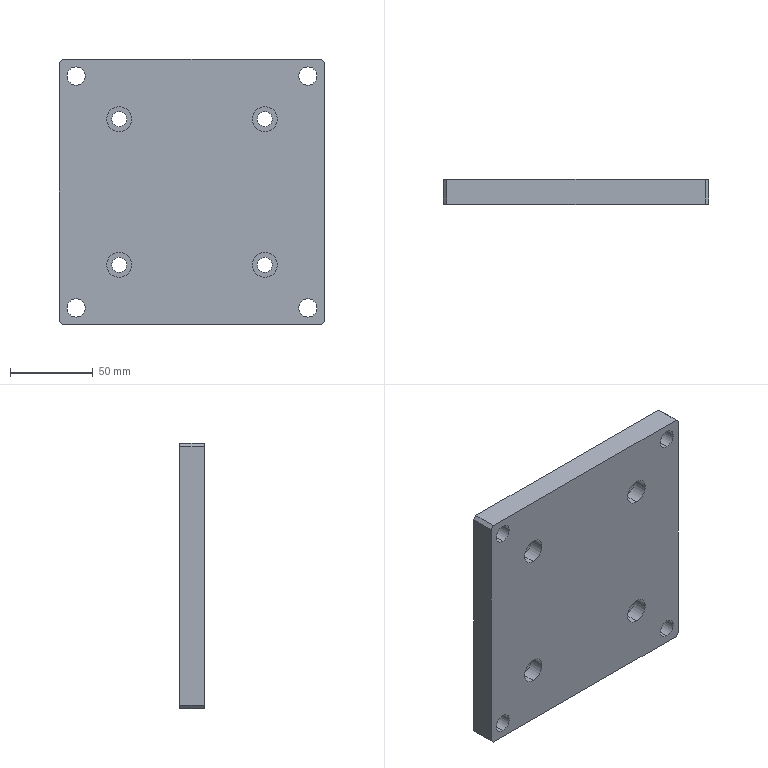Part | SolidWorks | features HoleWzd 2, Chamfer 1, Extrusion 1 | 1 solid | 38 faces | box 160 x 15 x 160 mm | volume 370289 mm3 | cylinder 24 | plane 14 | commonest cylinder face diameters 9 x8 11 x8 15 x8
STEP:
#1=CARTESIAN_POINT('',(70.,-7.5,64.5));
#2=VERTEX_POINT('',#1);
#3=CARTESIAN_POINT('',(70.,-7.5,75.5));
#4=VERTEX_POINT('',#3);
#5=CARTESIAN_POINT('',(70.,-7.5,70.));
#6=DIRECTION('',(0.,1.,0.));
#7=DIRECTION('',(0.,0.,1.));
#8=AXIS2_PLACEMENT_3D('',#5,#6,#7);
#9=CIRCLE('',#8,5.5);
#10=EDGE_CURVE('',#2,#4,#9,.T.);
#11=ORIENTED_EDGE('',*,*,#10,.F.);
#12=CARTESIAN_POINT('',(70.,7.5,64.5));
#13=VERTEX_POINT('',#12);
#14=CARTESIAN_POINT('',(70.,7.5,64.5));
#15=DIRECTION('',(0.,1.,0.));
#16=VECTOR('',#15,1000.);
#17=LINE('',#14,#16);
#18=EDGE_CURVE('',#2,#13,#17,.T.);
#19=ORIENTED_EDGE('',*,*,#18,.T.);
#20=CARTESIAN_POINT('',(70.,7.5,75.5));
#21=VERTEX_POINT('',#20);
#22=CARTESIAN_POINT('',(70.,7.5,70.));
#23=DIRECTION('',(0.,1.,0.));
#24=DIRECTION('',(0.,0.,1.));
#25=AXIS2_PLACEMENT_3D('',#22,#23,#24);
#26=CIRCLE('',#25,5.5);
#27=EDGE_CURVE('',#13,#21,#26,.T.);
#28=ORIENTED_EDGE('',*,*,#27,.T.);
#29=CARTESIAN_POINT('',(70.,7.5,75.5));
#30=DIRECTION('',(0.,1.,0.));
#31=VECTOR('',#30,1000.);
#32=LINE('',#29,#31);
#33=EDGE_CURVE('',#4,#21,#32,.T.);
#34=ORIENTED_EDGE('',*,*,#33,.F.);
#35=EDGE_LOOP('',(#11,#19,#28,#34));
#36=FACE_OUTER_BOUND('',#35,.T.);
#37=CARTESIAN_POINT('',(70.,7.5,70.));
#38=DIRECTION('',(0.,1.,0.));
#39=DIRECTION('',(0.,0.,1.));
#40=AXIS2_PLACEMENT_3D('',#37,#38,#39);
#41=CYLINDRICAL_SURFACE('',#40,5.5);
#42=ADVANCED_FACE('',(#36),#41,.F.);
#43=CARTESIAN_POINT('',(70.,-7.5,-75.5));
#44=VERTEX_POINT('',#43);
#45=CARTESIAN_POINT('',(70.,-7.5,-64.5));
#46=VERTEX_POINT('',#45);
#47=CARTESIAN_POINT('',(70.,-7.5,-70.));
#48=DIRECTION('',(0.,1.,0.));
#49=DIRECTION('',(0.,0.,1.));
#50=AXIS2_PLACEMENT_3D('',#47,#48,#49);
#51=CIRCLE('',#50,5.5);
#52=EDGE_CURVE('',#44,#46,#51,.T.);
#53=ORIENTED_EDGE('',*,*,#52,.F.);
#54=CARTESIAN_POINT('',(70.,7.5,-75.5));
#55=VERTEX_POINT('',#54);
#56=CARTESIAN_POINT('',(70.,7.5,-75.5));
#57=DIRECTION('',(0.,1.,0.));
#58=VECTOR('',#57,1000.);
#59=LINE('',#56,#58);
#60=EDGE_CURVE('',#44,#55,#59,.T.);
#61=ORIENTED_EDGE('',*,*,#60,.T.);
#62=CARTESIAN_POINT('',(70.,7.5,-64.5));
#63=VERTEX_POINT('',#62);
#64=CARTESIAN_POINT('',(70.,7.5,-70.));
#65=DIRECTION('',(0.,1.,0.));
#66=DIRECTION('',(0.,0.,1.));
#67=AXIS2_PLACEMENT_3D('',#64,#65,#66);
#68=CIRCLE('',#67,5.5);
#69=EDGE_CURVE('',#55,#63,#68,.T.);
#70=ORIENTED_EDGE('',*,*,#69,.T.);
#71=CARTESIAN_POINT('',(70.,7.5,-64.5));
#72=DIRECTION('',(0.,1.,0.));
#73=VECTOR('',#72,1000.);
#74=LINE('',#71,#73);
#75=EDGE_CURVE('',#46,#63,#74,.T.);
#76=ORIENTED_EDGE('',*,*,#75,.F.);
#77=EDGE_LOOP('',(#53,#61,#70,#76));
#78=FACE_OUTER_BOUND('',#77,.T.);
#79=CARTESIAN_POINT('',(70.,7.5,-70.));
#80=DIRECTION('',(0.,1.,0.));
#81=DIRECTION('',(0.,0.,1.));
#82=AXIS2_PLACEMENT_3D('',#79,#80,#81);
#83=CYLINDRICAL_SURFACE('',#82,5.5);
#84=ADVANCED_FACE('',(#78),#83,.F.);
#85=CARTESIAN_POINT('',(-70.,-7.5,-75.5));
#86=VERTEX_POINT('',#85);
#87=CARTESIAN_POINT('',(-70.,-7.5,-64.5));
#88=VERTEX_POINT('',#87);
#89=CARTESIAN_POINT('',(-70.,-7.5,-70.));
#90=DIRECTION('',(0.,1.,0.));
#91=DIRECTION('',(0.,0.,1.));
#92=AXIS2_PLACEMENT_3D('',#89,#90,#91);
#93=CIRCLE('',#92,5.5);
#94=EDGE_CURVE('',#86,#88,#93,.T.);
#95=ORIENTED_EDGE('',*,*,#94,.F.);
#96=CARTESIAN_POINT('',(-70.,7.5,-75.5));
#97=VERTEX_POINT('',#96);
#98=CARTESIAN_POINT('',(-70.,7.5,-75.5));
#99=DIRECTION('',(0.,1.,0.));
#100=VECTOR('',#99,1000.);
#101=LINE('',#98,#100);
#102=EDGE_CURVE('',#86,#97,#101,.T.);
#103=ORIENTED_EDGE('',*,*,#102,.T.);
#104=CARTESIAN_POINT('',(-70.,7.5,-64.5));
#105=VERTEX_POINT('',#104);
#106=CARTESIAN_POINT('',(-70.,7.5,-70.));
#107=DIRECTION('',(0.,1.,0.));
#108=DIRECTION('',(0.,0.,1.));
#109=AXIS2_PLACEMENT_3D('',#106,#107,#108);
#110=CIRCLE('',#109,5.5);
#111=EDGE_CURVE('',#97,#105,#110,.T.);
#112=ORIENTED_EDGE('',*,*,#111,.T.);
#113=CARTESIAN_POINT('',(-70.,7.5,-64.5));
#114=DIRECTION('',(0.,1.,0.));
#115=VECTOR('',#114,1000.);
#116=LINE('',#113,#115);
#117=EDGE_CURVE('',#88,#105,#116,.T.);
#118=ORIENTED_EDGE('',*,*,#117,.F.);
#119=EDGE_LOOP('',(#95,#103,#112,#118));
#120=FACE_OUTER_BOUND('',#119,.T.);
#121=CARTESIAN_POINT('',(-70.,7.5,-70.));
#122=DIRECTION('',(0.,1.,0.));
#123=DIRECTION('',(0.,0.,1.));
#124=AXIS2_PLACEMENT_3D('',#121,#122,#123);
#125=CYLINDRICAL_SURFACE('',#124,5.5);
#126=ADVANCED_FACE('',(#120),#125,.F.);
#127=CARTESIAN_POINT('',(-70.,-7.5,64.5));
#128=VERTEX_POINT('',#127);
#129=CARTESIAN_POINT('',(-70.,-7.5,75.5));
#130=VERTEX_POINT('',#129);
#131=CARTESIAN_POINT('',(-70.,-7.5,70.));
#132=DIRECTION('',(0.,1.,0.));
#133=DIRECTION('',(0.,0.,1.));
#134=AXIS2_PLACEMENT_3D('',#131,#132,#133);
#135=CIRCLE('',#134,5.5);
#136=EDGE_CURVE('',#128,#130,#135,.T.);
#137=ORIENTED_EDGE('',*,*,#136,.F.);
#138=CARTESIAN_POINT('',(-70.,7.5,64.5));
#139=VERTEX_POINT('',#138);
#140=CARTESIAN_POINT('',(-70.,7.5,64.5));
#141=DIRECTION('',(0.,1.,0.));
#142=VECTOR('',#141,1000.);
#143=LINE('',#140,#142);
#144=EDGE_CURVE('',#128,#139,#143,.T.);
#145=ORIENTED_EDGE('',*,*,#144,.T.);
#146=CARTESIAN_POINT('',(-70.,7.5,75.5));
#147=VERTEX_POINT('',#146);
#148=CARTESIAN_POINT('',(-70.,7.5,70.));
#149=DIRECTION('',(0.,1.,0.));
#150=DIRECTION('',(0.,0.,1.));
#151=AXIS2_PLACEMENT_3D('',#148,#149,#150);
#152=CIRCLE('',#151,5.5);
#153=EDGE_CURVE('',#139,#147,#152,.T.);
#154=ORIENTED_EDGE('',*,*,#153,.T.);
#155=CARTESIAN_POINT('',(-70.,7.5,75.5));
#156=DIRECTION('',(0.,1.,0.));
#157=VECTOR('',#156,1000.);
#158=LINE('',#155,#157);
#159=EDGE_CURVE('',#130,#147,#158,.T.);
#160=ORIENTED_EDGE('',*,*,#159,.F.);
#161=EDGE_LOOP('',(#137,#145,#154,#160));
#162=FACE_OUTER_BOUND('',#161,.T.);
#163=CARTESIAN_POINT('',(-70.,7.5,70.));
#164=DIRECTION('',(0.,1.,0.));
#165=DIRECTION('',(0.,0.,1.));
#166=AXIS2_PLACEMENT_3D('',#163,#164,#165);
#167=CYLINDRICAL_SURFACE('',#166,5.5);
#168=ADVANCED_FACE('',(#162),#167,.F.);
#169=CARTESIAN_POINT('',(-44.,1.5,51.5));
#170=VERTEX_POINT('',#169);
#171=CARTESIAN_POINT('',(-44.,1.5,36.5));
#172=VERTEX_POINT('',#171);
#173=CARTESIAN_POINT('',(-44.,1.5,44.));
#174=DIRECTION('',(0.,-1.,0.));
#175=DIRECTION('',(0.,0.,-1.));
#176=AXIS2_PLACEMENT_3D('',#173,#174,#175);
#177=CIRCLE('',#176,7.5);
#178=EDGE_CURVE('',#170,#172,#177,.T.);
#179=ORIENTED_EDGE('',*,*,#178,.F.);
#180=CARTESIAN_POINT('',(-44.,-7.5,51.5));
#181=VERTEX_POINT('',#180);
#182=CARTESIAN_POINT('',(-44.,-7.5,51.5));
#183=DIRECTION('',(0.,-1.,0.));
#184=VECTOR('',#183,1000.);
#185=LINE('',#182,#184);
#186=EDGE_CURVE('',#170,#181,#185,.T.);
#187=ORIENTED_EDGE('',*,*,#186,.T.);
#188=CARTESIAN_POINT('',(-44.,-7.5,36.5));
#189=VERTEX_POINT('',#188);
#190=CARTESIAN_POINT('',(-44.,-7.5,44.));
#191=DIRECTION('',(0.,-1.,0.));
#192=DIRECTION('',(0.,0.,-1.));
#193=AXIS2_PLACEMENT_3D('',#190,#191,#192);
#194=CIRCLE('',#193,7.5);
#195=EDGE_CURVE('',#181,#189,#194,.T.);
#196=ORIENTED_EDGE('',*,*,#195,.T.);
#197=CARTESIAN_POINT('',(-44.,-7.5,36.5));
#198=DIRECTION('',(0.,-1.,0.));
#199=VECTOR('',#198,1000.);
#200=LINE('',#197,#199);
#201=EDGE_CURVE('',#172,#189,#200,.T.);
#202=ORIENTED_EDGE('',*,*,#201,.F.);
#203=EDGE_LOOP('',(#179,#187,#196,#202));
#204=FACE_OUTER_BOUND('',#203,.T.);
#205=CARTESIAN_POINT('',(-44.,-7.5,44.));
#206=DIRECTION('',(0.,-1.,0.));
#207=DIRECTION('',(0.,0.,-1.));
#208=AXIS2_PLACEMENT_3D('',#205,#206,#207);
#209=CYLINDRICAL_SURFACE('',#208,7.5);
#210=ADVANCED_FACE('',(#204),#209,.F.);
#211=CARTESIAN_POINT('',(-44.,7.5,48.5));
#212=VERTEX_POINT('',#211);
#213=CARTESIAN_POINT('',(-44.,7.5,39.5));
#214=VERTEX_POINT('',#213);
#215=CARTESIAN_POINT('',(-44.,7.5,44.));
#216=DIRECTION('',(0.,-1.,0.));
#217=DIRECTION('',(0.,0.,-1.));
#218=AXIS2_PLACEMENT_3D('',#215,#216,#217);
#219=CIRCLE('',#218,4.5);
#220=EDGE_CURVE('',#212,#214,#219,.T.);
#221=ORIENTED_EDGE('',*,*,#220,.F.);
#222=CARTESIAN_POINT('',(-44.,1.5,48.5));
#223=VERTEX_POINT('',#222);
#224=CARTESIAN_POINT('',(-44.,-7.5,48.5));
#225=DIRECTION('',(0.,-1.,0.));
#226=VECTOR('',#225,1000.);
#227=LINE('',#224,#226);
#228=EDGE_CURVE('',#212,#223,#227,.T.);
#229=ORIENTED_EDGE('',*,*,#228,.T.);
#230=CARTESIAN_POINT('',(-44.,1.5,39.5));
#231=VERTEX_POINT('',#230);
#232=CARTESIAN_POINT('',(-44.,1.5,44.));
#233=DIRECTION('',(0.,-1.,0.));
#234=DIRECTION('',(0.,0.,-1.));
#235=AXIS2_PLACEMENT_3D('',#232,#233,#234);
#236=CIRCLE('',#235,4.5);
#237=EDGE_CURVE('',#223,#231,#236,.T.);
#238=ORIENTED_EDGE('',*,*,#237,.T.);
#239=CARTESIAN_POINT('',(-44.,-7.5,39.5));
#240=DIRECTION('',(0.,-1.,0.));
#241=VECTOR('',#240,1000.);
#242=LINE('',#239,#241);
#243=EDGE_CURVE('',#214,#231,#242,.T.);
#244=ORIENTED_EDGE('',*,*,#243,.F.);
#245=EDGE_LOOP('',(#221,#229,#238,#244));
#246=FACE_OUTER_BOUND('',#245,.T.);
#247=CARTESIAN_POINT('',(-44.,-7.5,44.));
#248=DIRECTION('',(0.,-1.,0.));
#249=DIRECTION('',(0.,0.,-1.));
#250=AXIS2_PLACEMENT_3D('',#247,#248,#249);
#251=CYLINDRICAL_SURFACE('',#250,4.5);
#252=ADVANCED_FACE('',(#246),#251,.F.);
#253=CARTESIAN_POINT('',(-44.,1.5,-36.5));
#254=VERTEX_POINT('',#253);
#255=CARTESIAN_POINT('',(-44.,1.5,-51.5));
#256=VERTEX_POINT('',#255);
#257=CARTESIAN_POINT('',(-44.,1.5,-44.));
#258=DIRECTION('',(0.,-1.,0.));
#259=DIRECTION('',(0.,0.,-1.));
#260=AXIS2_PLACEMENT_3D('',#257,#258,#259);
#261=CIRCLE('',#260,7.5);
#262=EDGE_CURVE('',#254,#256,#261,.T.);
#263=ORIENTED_EDGE('',*,*,#262,.F.);
#264=CARTESIAN_POINT('',(-44.,-7.5,-36.5));
#265=VERTEX_POINT('',#264);
#266=CARTESIAN_POINT('',(-44.,-7.5,-36.5));
#267=DIRECTION('',(0.,-1.,0.));
#268=VECTOR('',#267,1000.);
#269=LINE('',#266,#268);
#270=EDGE_CURVE('',#254,#265,#269,.T.);
#271=ORIENTED_EDGE('',*,*,#270,.T.);
#272=CARTESIAN_POINT('',(-44.,-7.5,-51.5));
#273=VERTEX_POINT('',#272);
#274=CARTESIAN_POINT('',(-44.,-7.5,-44.));
#275=DIRECTION('',(0.,-1.,0.));
#276=DIRECTION('',(0.,0.,-1.));
#277=AXIS2_PLACEMENT_3D('',#274,#275,#276);
#278=CIRCLE('',#277,7.5);
#279=EDGE_CURVE('',#265,#273,#278,.T.);
#280=ORIENTED_EDGE('',*,*,#279,.T.);
#281=CARTESIAN_POINT('',(-44.,-7.5,-51.5));
#282=DIRECTION('',(0.,-1.,0.));
#283=VECTOR('',#282,1000.);
#284=LINE('',#281,#283);
#285=EDGE_CURVE('',#256,#273,#284,.T.);
#286=ORIENTED_EDGE('',*,*,#285,.F.);
#287=EDGE_LOOP('',(#263,#271,#280,#286));
#288=FACE_OUTER_BOUND('',#287,.T.);
#289=CARTESIAN_POINT('',(-44.,-7.5,-44.));
#290=DIRECTION('',(0.,-1.,0.));
#291=DIRECTION('',(0.,0.,-1.));
#292=AXIS2_PLACEMENT_3D('',#289,#290,#291);
#293=CYLINDRICAL_SURFACE('',#292,7.5);
#294=ADVANCED_FACE('',(#288),#293,.F.);
#295=CARTESIAN_POINT('',(-44.,7.5,-39.5));
#296=VERTEX_POINT('',#295);
#297=CARTESIAN_POINT('',(-44.,7.5,-48.5));
#298=VERTEX_POINT('',#297);
#299=CARTESIAN_POINT('',(-44.,7.5,-44.));
#300=DIRECTION('',(0.,-1.,0.));
#301=DIRECTION('',(0.,0.,-1.));
#302=AXIS2_PLACEMENT_3D('',#299,#300,#301);
#303=CIRCLE('',#302,4.5);
#304=EDGE_CURVE('',#296,#298,#303,.T.);
#305=ORIENTED_EDGE('',*,*,#304,.F.);
#306=CARTESIAN_POINT('',(-44.,1.5,-39.5));
#307=VERTEX_POINT('',#306);
#308=CARTESIAN_POINT('',(-44.,-7.5,-39.5));
#309=DIRECTION('',(0.,-1.,0.));
#310=VECTOR('',#309,1000.);
#311=LINE('',#308,#310);
#312=EDGE_CURVE('',#296,#307,#311,.T.);
#313=ORIENTED_EDGE('',*,*,#312,.T.);
#314=CARTESIAN_POINT('',(-44.,1.5,-48.5));
#315=VERTEX_POINT('',#314);
#316=CARTESIAN_POINT('',(-44.,1.5,-44.));
#317=DIRECTION('',(0.,-1.,0.));
#318=DIRECTION('',(0.,0.,-1.));
#319=AXIS2_PLACEMENT_3D('',#316,#317,#318);
#320=CIRCLE('',#319,4.5);
#321=EDGE_CURVE('',#307,#315,#320,.T.);
#322=ORIENTED_EDGE('',*,*,#321,.T.);
#323=CARTESIAN_POINT('',(-44.,-7.5,-48.5));
#324=DIRECTION('',(0.,-1.,0.));
#325=VECTOR('',#324,1000.);
#326=LINE('',#323,#325);
#327=EDGE_CURVE('',#298,#315,#326,.T.);
#328=ORIENTED_EDGE('',*,*,#327,.F.);
#329=EDGE_LOOP('',(#305,#313,#322,#328));
#330=FACE_OUTER_BOUND('',#329,.T.);
#331=CARTESIAN_POINT('',(-44.,-7.5,-44.));
#332=DIRECTION('',(0.,-1.,0.));
#333=DIRECTION('',(0.,0.,-1.));
#334=AXIS2_PLACEMENT_3D('',#331,#332,#333);
#335=CYLINDRICAL_SURFACE('',#334,4.5);
#336=ADVANCED_FACE('',(#330),#335,.F.);
#337=CARTESIAN_POINT('',(44.,1.5,-36.5));
#338=VERTEX_POINT('',#337);
#339=CARTESIAN_POINT('',(44.,1.5,-51.5));
#340=VERTEX_POINT('',#339);
#341=CARTESIAN_POINT('',(44.,1.5,-44.));
#342=DIRECTION('',(0.,-1.,0.));
#343=DIRECTION('',(0.,0.,-1.));
#344=AXIS2_PLACEMENT_3D('',#341,#342,#343);
#345=CIRCLE('',#344,7.5);
#346=EDGE_CURVE('',#338,#340,#345,.T.);
#347=ORIENTED_EDGE('',*,*,#346,.F.);
#348=CARTESIAN_POINT('',(44.,-7.5,-36.5));
#349=VERTEX_POINT('',#348);
#350=CARTESIAN_POINT('',(44.,-7.5,-36.5));
#351=DIRECTION('',(0.,-1.,0.));
#352=VECTOR('',#351,1000.);
#353=LINE('',#350,#352);
#354=EDGE_CURVE('',#338,#349,#353,.T.);
#355=ORIENTED_EDGE('',*,*,#354,.T.);
#356=CARTESIAN_POINT('',(44.,-7.5,-51.5));
#357=VERTEX_POINT('',#356);
#358=CARTESIAN_POINT('',(44.,-7.5,-44.));
#359=DIRECTION('',(0.,-1.,0.));
#360=DIRECTION('',(0.,0.,-1.));
#361=AXIS2_PLACEMENT_3D('',#358,#359,#360);
#362=CIRCLE('',#361,7.5);
#363=EDGE_CURVE('',#349,#357,#362,.T.);
#364=ORIENTED_EDGE('',*,*,#363,.T.);
#365=CARTESIAN_POINT('',(44.,-7.5,-51.5));
#366=DIRECTION('',(0.,-1.,0.));
#367=VECTOR('',#366,1000.);
#368=LINE('',#365,#367);
#369=EDGE_CURVE('',#340,#357,#368,.T.);
#370=ORIENTED_EDGE('',*,*,#369,.F.);
#371=EDGE_LOOP('',(#347,#355,#364,#370));
#372=FACE_OUTER_BOUND('',#371,.T.);
#373=CARTESIAN_POINT('',(44.,-7.5,-44.));
#374=DIRECTION('',(0.,-1.,0.));
#375=DIRECTION('',(0.,0.,-1.));
#376=AXIS2_PLACEMENT_3D('',#373,#374,#375);
#377=CYLINDRICAL_SURFACE('',#376,7.5);
#378=ADVANCED_FACE('',(#372),#377,.F.);
#379=CARTESIAN_POINT('',(44.,7.5,-39.5));
#380=VERTEX_POINT('',#379);
#381=CARTESIAN_POINT('',(44.,7.5,-48.5));
#382=VERTEX_POINT('',#381);
#383=CARTESIAN_POINT('',(44.,7.5,-44.));
#384=DIRECTION('',(0.,-1.,0.));
#385=DIRECTION('',(0.,0.,-1.));
#386=AXIS2_PLACEMENT_3D('',#383,#384,#385);
#387=CIRCLE('',#386,4.5);
#388=EDGE_CURVE('',#380,#382,#387,.T.);
#389=ORIENTED_EDGE('',*,*,#388,.F.);
#390=CARTESIAN_POINT('',(44.,1.5,-39.5));
#391=VERTEX_POINT('',#390);
#392=CARTESIAN_POINT('',(44.,-7.5,-39.5));
#393=DIRECTION('',(0.,-1.,0.));
#394=VECTOR('',#393,1000.);
#395=LINE('',#392,#394);
#396=EDGE_CURVE('',#380,#391,#395,.T.);
#397=ORIENTED_EDGE('',*,*,#396,.T.);
#398=CARTESIAN_POINT('',(44.,1.5,-48.5));
#399=VERTEX_POINT('',#398);
#400=CARTESIAN_POINT('',(44.,1.5,-44.));
#401=DIRECTION('',(0.,-1.,0.));
#402=DIRECTION('',(0.,0.,-1.));
#403=AXIS2_PLACEMENT_3D('',#400,#401,#402);
#404=CIRCLE('',#403,4.5);
#405=EDGE_CURVE('',#391,#399,#404,.T.);
#406=ORIENTED_EDGE('',*,*,#405,.T.);
#407=CARTESIAN_POINT('',(44.,-7.5,-48.5));
#408=DIRECTION('',(0.,-1.,0.));
#409=VECTOR('',#408,1000.);
#410=LINE('',#407,#409);
#411=EDGE_CURVE('',#382,#399,#410,.T.);
#412=ORIENTED_EDGE('',*,*,#411,.F.);
#413=EDGE_LOOP('',(#389,#397,#406,#412));
#414=FACE_OUTER_BOUND('',#413,.T.);
#415=CARTESIAN_POINT('',(44.,-7.5,-44.));
#416=DIRECTION('',(0.,-1.,0.));
#417=DIRECTION('',(0.,0.,-1.));
#418=AXIS2_PLACEMENT_3D('',#415,#416,#417);
#419=CYLINDRICAL_SURFACE('',#418,4.5);
#420=ADVANCED_FACE('',(#414),#419,.F.);
#421=CARTESIAN_POINT('',(44.,1.5,51.5));
#422=VERTEX_POINT('',#421);
#423=CARTESIAN_POINT('',(44.,1.5,36.5));
#424=VERTEX_POINT('',#423);
#425=CARTESIAN_POINT('',(44.,1.5,44.));
#426=DIRECTION('',(0.,-1.,0.));
#427=DIRECTION('',(0.,0.,-1.));
#428=AXIS2_PLACEMENT_3D('',#425,#426,#427);
#429=CIRCLE('',#428,7.5);
#430=EDGE_CURVE('',#422,#424,#429,.T.);
#431=ORIENTED_EDGE('',*,*,#430,.F.);
#432=CARTESIAN_POINT('',(44.,-7.5,51.5));
#433=VERTEX_POINT('',#432);
#434=CARTESIAN_POINT('',(44.,-7.5,51.5));
#435=DIRECTION('',(0.,-1.,0.));
#436=VECTOR('',#435,1000.);
#437=LINE('',#434,#436);
#438=EDGE_CURVE('',#422,#433,#437,.T.);
#439=ORIENTED_EDGE('',*,*,#438,.T.);
#440=CARTESIAN_POINT('',(44.,-7.5,36.5));
#441=VERTEX_POINT('',#440);
#442=CARTESIAN_POINT('',(44.,-7.5,44.));
#443=DIRECTION('',(0.,-1.,0.));
#444=DIRECTION('',(0.,0.,-1.));
#445=AXIS2_PLACEMENT_3D('',#442,#443,#444);
#446=CIRCLE('',#445,7.5);
#447=EDGE_CURVE('',#433,#441,#446,.T.);
#448=ORIENTED_EDGE('',*,*,#447,.T.);
#449=CARTESIAN_POINT('',(44.,-7.5,36.5));
#450=DIRECTION('',(0.,-1.,0.));
#451=VECTOR('',#450,1000.);
#452=LINE('',#449,#451);
#453=EDGE_CURVE('',#424,#441,#452,.T.);
#454=ORIENTED_EDGE('',*,*,#453,.F.);
#455=EDGE_LOOP('',(#431,#439,#448,#454));
#456=FACE_OUTER_BOUND('',#455,.T.);
#457=CARTESIAN_POINT('',(44.,-7.5,44.));
#458=DIRECTION('',(0.,-1.,0.));
#459=DIRECTION('',(0.,0.,-1.));
#460=AXIS2_PLACEMENT_3D('',#457,#458,#459);
#461=CYLINDRICAL_SURFACE('',#460,7.5);
#462=ADVANCED_FACE('',(#456),#461,.F.);
#463=CARTESIAN_POINT('',(44.,7.5,48.5));
#464=VERTEX_POINT('',#463);
#465=CARTESIAN_POINT('',(44.,7.5,39.5));
#466=VERTEX_POINT('',#465);
#467=CARTESIAN_POINT('',(44.,7.5,44.));
#468=DIRECTION('',(0.,-1.,0.));
#469=DIRECTION('',(0.,0.,-1.));
#470=AXIS2_PLACEMENT_3D('',#467,#468,#469);
#471=CIRCLE('',#470,4.5);
#472=EDGE_CURVE('',#464,#466,#471,.T.);
#473=ORIENTED_EDGE('',*,*,#472,.F.);
#474=CARTESIAN_POINT('',(44.,1.5,48.5));
#475=VERTEX_POINT('',#474);
#476=CARTESIAN_POINT('',(44.,-7.5,48.5));
#477=DIRECTION('',(0.,-1.,0.));
#478=VECTOR('',#477,1000.);
#479=LINE('',#476,#478);
#480=EDGE_CURVE('',#464,#475,#479,.T.);
#481=ORIENTED_EDGE('',*,*,#480,.T.);
#482=CARTESIAN_POINT('',(44.,1.5,39.5));
#483=VERTEX_POINT('',#482);
#484=CARTESIAN_POINT('',(44.,1.5,44.));
#485=DIRECTION('',(0.,-1.,0.));
#486=DIRECTION('',(0.,0.,-1.));
#487=AXIS2_PLACEMENT_3D('',#484,#485,#486);
#488=CIRCLE('',#487,4.5);
#489=EDGE_CURVE('',#475,#483,#488,.T.);
#490=ORIENTED_EDGE('',*,*,#489,.T.);
#491=CARTESIAN_POINT('',(44.,-7.5,39.5));
#492=DIRECTION('',(0.,-1.,0.));
#493=VECTOR('',#492,1000.);
#494=LINE('',#491,#493);
#495=EDGE_CURVE('',#466,#483,#494,.T.);
#496=ORIENTED_EDGE('',*,*,#495,.F.);
#497=EDGE_LOOP('',(#473,#481,#490,#496));
#498=FACE_OUTER_BOUND('',#497,.T.);
#499=CARTESIAN_POINT('',(44.,-7.5,44.));
#500=DIRECTION('',(0.,-1.,0.));
#501=DIRECTION('',(0.,0.,-1.));
#502=AXIS2_PLACEMENT_3D('',#499,#500,#501);
#503=CYLINDRICAL_SURFACE('',#502,4.5);
#504=ADVANCED_FACE('',(#498),#503,.F.);
#505=CARTESIAN_POINT('',(80.,7.5,78.));
#506=VERTEX_POINT('',#505);
#507=CARTESIAN_POINT('',(80.,7.5,-78.));
#508=VERTEX_POINT('',#507);
#509=CARTESIAN_POINT('',(80.,7.5,80.));
#510=DIRECTION('',(0.,0.,-1.));
#511=VECTOR('',#510,1000.);
#512=LINE('',#509,#511);
#513=EDGE_CURVE('',#506,#508,#512,.T.);
#514=ORIENTED_EDGE('',*,*,#513,.F.);
#515=CARTESIAN_POINT('',(80.,-7.5,78.));
#516=VERTEX_POINT('',#515);
#517=CARTESIAN_POINT('',(80.,7.5,78.));
#518=DIRECTION('',(0.,-1.,0.));
#519=VECTOR('',#518,1000.);
#520=LINE('',#517,#519);
#521=EDGE_CURVE('',#506,#516,#520,.T.);
#522=ORIENTED_EDGE('',*,*,#521,.T.);
#523=CARTESIAN_POINT('',(80.,-7.5,-78.));
#524=VERTEX_POINT('',#523);
#525=CARTESIAN_POINT('',(80.,-7.5,80.));
#526=DIRECTION('',(0.,0.,-1.));
#527=VECTOR('',#526,1000.);
#528=LINE('',#525,#527);
#529=EDGE_CURVE('',#516,#524,#528,.T.);
#530=ORIENTED_EDGE('',*,*,#529,.T.);
#531=CARTESIAN_POINT('',(80.,7.5,-78.));
#532=DIRECTION('',(0.,1.,0.));
#533=VECTOR('',#532,1000.);
#534=LINE('',#531,#533);
#535=EDGE_CURVE('',#524,#508,#534,.T.);
#536=ORIENTED_EDGE('',*,*,#535,.T.);
#537=EDGE_LOOP('',(#514,#522,#530,#536));
#538=FACE_OUTER_BOUND('',#537,.T.);
#539=CARTESIAN_POINT('',(80.,7.5,80.));
#540=DIRECTION('',(-1.,0.,0.));
#541=DIRECTION('',(0.,0.,1.));
#542=AXIS2_PLACEMENT_3D('',#539,#540,#541);
#543=PLANE('',#542);
#544=ADVANCED_FACE('',(#538),#543,.F.);
#545=CARTESIAN_POINT('',(78.,7.5,-80.));
#546=VERTEX_POINT('',#545);
#547=CARTESIAN_POINT('',(-78.,7.5,-80.));
#548=VERTEX_POINT('',#547);
#549=CARTESIAN_POINT('',(-80.,7.5,-80.));
#550=DIRECTION('',(-1.,0.,0.));
#551=VECTOR('',#550,1000.);
#552=LINE('',#549,#551);
#553=EDGE_CURVE('',#546,#548,#552,.T.);
#554=ORIENTED_EDGE('',*,*,#553,.F.);
#555=CARTESIAN_POINT('',(78.,-7.5,-80.));
#556=VERTEX_POINT('',#555);
#557=CARTESIAN_POINT('',(78.,7.5,-80.));
#558=DIRECTION('',(0.,-1.,0.));
#559=VECTOR('',#558,1000.);
#560=LINE('',#557,#559);
#561=EDGE_CURVE('',#546,#556,#560,.T.);
#562=ORIENTED_EDGE('',*,*,#561,.T.);
#563=CARTESIAN_POINT('',(-78.,-7.5,-80.));
#564=VERTEX_POINT('',#563);
#565=CARTESIAN_POINT('',(-80.,-7.5,-80.));
#566=DIRECTION('',(-1.,0.,0.));
#567=VECTOR('',#566,1000.);
#568=LINE('',#565,#567);
#569=EDGE_CURVE('',#556,#564,#568,.T.);
#570=ORIENTED_EDGE('',*,*,#569,.T.);
#571=CARTESIAN_POINT('',(-78.,7.5,-80.));
#572=DIRECTION('',(0.,1.,0.));
#573=VECTOR('',#572,1000.);
#574=LINE('',#571,#573);
#575=EDGE_CURVE('',#564,#548,#574,.T.);
#576=ORIENTED_EDGE('',*,*,#575,.T.);
#577=EDGE_LOOP('',(#554,#562,#570,#576));
#578=FACE_OUTER_BOUND('',#577,.T.);
#579=CARTESIAN_POINT('',(-80.,7.5,-80.));
#580=DIRECTION('',(0.,0.,1.));
#581=DIRECTION('',(1.,0.,0.));
#582=AXIS2_PLACEMENT_3D('',#579,#580,#581);
#583=PLANE('',#582);
#584=ADVANCED_FACE('',(#578),#583,.F.);
#585=CARTESIAN_POINT('',(-80.,7.5,-78.));
#586=VERTEX_POINT('',#585);
#587=CARTESIAN_POINT('',(-80.,7.5,78.));
#588=VERTEX_POINT('',#587);
#589=CARTESIAN_POINT('',(-80.,7.5,80.));
#590=DIRECTION('',(0.,0.,1.));
#591=VECTOR('',#590,1000.);
#592=LINE('',#589,#591);
#593=EDGE_CURVE('',#586,#588,#592,.T.);
#594=ORIENTED_EDGE('',*,*,#593,.F.);
#595=CARTESIAN_POINT('',(-80.,-7.5,-78.));
#596=VERTEX_POINT('',#595);
#597=CARTESIAN_POINT('',(-80.,7.5,-78.));
#598=DIRECTION('',(0.,-1.,0.));
#599=VECTOR('',#598,1000.);
#600=LINE('',#597,#599);
#601=EDGE_CURVE('',#586,#596,#600,.T.);
#602=ORIENTED_EDGE('',*,*,#601,.T.);
#603=CARTESIAN_POINT('',(-80.,-7.5,78.));
#604=VERTEX_POINT('',#603);
#605=CARTESIAN_POINT('',(-80.,-7.5,80.));
#606=DIRECTION('',(0.,0.,1.));
#607=VECTOR('',#606,1000.);
#608=LINE('',#605,#607);
#609=EDGE_CURVE('',#596,#604,#608,.T.);
#610=ORIENTED_EDGE('',*,*,#609,.T.);
#611=CARTESIAN_POINT('',(-80.,7.5,78.));
#612=DIRECTION('',(0.,1.,0.));
#613=VECTOR('',#612,1000.);
#614=LINE('',#611,#613);
#615=EDGE_CURVE('',#604,#588,#614,.T.);
#616=ORIENTED_EDGE('',*,*,#615,.T.);
#617=EDGE_LOOP('',(#594,#602,#610,#616));
#618=FACE_OUTER_BOUND('',#617,.T.);
#619=CARTESIAN_POINT('',(-80.,7.5,80.));
#620=DIRECTION('',(1.,0.,0.));
#621=DIRECTION('',(0.,0.,-1.));
#622=AXIS2_PLACEMENT_3D('',#619,#620,#621);
#623=PLANE('',#622);
#624=ADVANCED_FACE('',(#618),#623,.F.);
#625=CARTESIAN_POINT('',(-78.,-7.5,80.));
#626=VERTEX_POINT('',#625);
#627=CARTESIAN_POINT('',(78.,-7.5,80.));
#628=VERTEX_POINT('',#627);
#629=CARTESIAN_POINT('',(-80.,-7.5,80.));
#630=DIRECTION('',(1.,0.,0.));
#631=VECTOR('',#630,1000.);
#632=LINE('',#629,#631);
#633=EDGE_CURVE('',#626,#628,#632,.T.);
#634=ORIENTED_EDGE('',*,*,#633,.T.);
#635=CARTESIAN_POINT('',(78.,7.5,80.));
#636=VERTEX_POINT('',#635);
#637=CARTESIAN_POINT('',(78.,7.5,80.));
#638=DIRECTION('',(0.,1.,0.));
#639=VECTOR('',#638,1000.);
#640=LINE('',#637,#639);
#641=EDGE_CURVE('',#628,#636,#640,.T.);
#642=ORIENTED_EDGE('',*,*,#641,.T.);
#643=CARTESIAN_POINT('',(-78.,7.5,80.));
#644=VERTEX_POINT('',#643);
#645=CARTESIAN_POINT('',(-80.,7.5,80.));
#646=DIRECTION('',(1.,0.,0.));
#647=VECTOR('',#646,1000.);
#648=LINE('',#645,#647);
#649=EDGE_CURVE('',#644,#636,#648,.T.);
#650=ORIENTED_EDGE('',*,*,#649,.F.);
#651=CARTESIAN_POINT('',(-78.,7.5,80.));
#652=DIRECTION('',(0.,-1.,0.));
#653=VECTOR('',#652,1000.);
#654=LINE('',#651,#653);
#655=EDGE_CURVE('',#644,#626,#654,.T.);
#656=ORIENTED_EDGE('',*,*,#655,.T.);
#657=EDGE_LOOP('',(#634,#642,#650,#656));
#658=FACE_OUTER_BOUND('',#657,.T.);
#659=CARTESIAN_POINT('',(-80.,7.5,80.));
#660=DIRECTION('',(0.,0.,-1.));
#661=DIRECTION('',(-1.,0.,0.));
#662=AXIS2_PLACEMENT_3D('',#659,#660,#661);
#663=PLANE('',#662);
#664=ADVANCED_FACE('',(#658),#663,.F.);
#665=CARTESIAN_POINT('',(70.,7.5,70.));
#666=DIRECTION('',(0.,1.,0.));
#667=DIRECTION('',(0.,0.,1.));
#668=AXIS2_PLACEMENT_3D('',#665,#666,#667);
#669=CIRCLE('',#668,5.5);
#670=EDGE_CURVE('',#21,#13,#669,.T.);
#671=ORIENTED_EDGE('',*,*,#670,.F.);
#672=ORIENTED_EDGE('',*,*,#27,.F.);
#673=EDGE_LOOP('',(#671,#672));
#674=FACE_BOUND('',#673,.T.);
#675=CARTESIAN_POINT('',(70.,7.5,-70.));
#676=DIRECTION('',(0.,1.,0.));
#677=DIRECTION('',(0.,0.,1.));
#678=AXIS2_PLACEMENT_3D('',#675,#676,#677);
#679=CIRCLE('',#678,5.5);
#680=EDGE_CURVE('',#63,#55,#679,.T.);
#681=ORIENTED_EDGE('',*,*,#680,.F.);
#682=ORIENTED_EDGE('',*,*,#69,.F.);
#683=EDGE_LOOP('',(#681,#682));
#684=FACE_BOUND('',#683,.T.);
#685=CARTESIAN_POINT('',(-70.,7.5,-70.));
#686=DIRECTION('',(0.,1.,0.));
#687=DIRECTION('',(0.,0.,1.));
#688=AXIS2_PLACEMENT_3D('',#685,#686,#687);
#689=CIRCLE('',#688,5.5);
#690=EDGE_CURVE('',#105,#97,#689,.T.);
#691=ORIENTED_EDGE('',*,*,#690,.F.);
#692=ORIENTED_EDGE('',*,*,#111,.F.);
#693=EDGE_LOOP('',(#691,#692));
#694=FACE_BOUND('',#693,.T.);
#695=CARTESIAN_POINT('',(-70.,7.5,70.));
#696=DIRECTION('',(0.,1.,0.));
#697=DIRECTION('',(0.,0.,1.));
#698=AXIS2_PLACEMENT_3D('',#695,#696,#697);
#699=CIRCLE('',#698,5.5);
#700=EDGE_CURVE('',#147,#139,#699,.T.);
#701=ORIENTED_EDGE('',*,*,#700,.F.);
#702=ORIENTED_EDGE('',*,*,#153,.F.);
#703=EDGE_LOOP('',(#701,#702));
#704=FACE_BOUND('',#703,.T.);
#705=CARTESIAN_POINT('',(-44.,7.5,44.));
#706=DIRECTION('',(0.,-1.,0.));
#707=DIRECTION('',(0.,0.,-1.));
#708=AXIS2_PLACEMENT_3D('',#705,#706,#707);
#709=CIRCLE('',#708,4.5);
#710=EDGE_CURVE('',#214,#212,#709,.T.);
#711=ORIENTED_EDGE('',*,*,#710,.T.);
#712=ORIENTED_EDGE('',*,*,#220,.T.);
#713=EDGE_LOOP('',(#711,#712));
#714=FACE_BOUND('',#713,.T.);
#715=CARTESIAN_POINT('',(-44.,7.5,-44.));
#716=DIRECTION('',(0.,-1.,0.));
#717=DIRECTION('',(0.,0.,-1.));
#718=AXIS2_PLACEMENT_3D('',#715,#716,#717);
#719=CIRCLE('',#718,4.5);
#720=EDGE_CURVE('',#298,#296,#719,.T.);
#721=ORIENTED_EDGE('',*,*,#720,.T.);
#722=ORIENTED_EDGE('',*,*,#304,.T.);
#723=EDGE_LOOP('',(#721,#722));
#724=FACE_BOUND('',#723,.T.);
#725=CARTESIAN_POINT('',(44.,7.5,-44.));
#726=DIRECTION('',(0.,-1.,0.));
#727=DIRECTION('',(0.,0.,-1.));
#728=AXIS2_PLACEMENT_3D('',#725,#726,#727);
#729=CIRCLE('',#728,4.5);
#730=EDGE_CURVE('',#382,#380,#729,.T.);
#731=ORIENTED_EDGE('',*,*,#730,.T.);
#732=ORIENTED_EDGE('',*,*,#388,.T.);
#733=EDGE_LOOP('',(#731,#732));
#734=FACE_BOUND('',#733,.T.);
#735=CARTESIAN_POINT('',(44.,7.5,44.));
#736=DIRECTION('',(0.,-1.,0.));
#737=DIRECTION('',(0.,0.,-1.));
#738=AXIS2_PLACEMENT_3D('',#735,#736,#737);
#739=CIRCLE('',#738,4.5);
#740=EDGE_CURVE('',#466,#464,#739,.T.);
#741=ORIENTED_EDGE('',*,*,#740,.T.);
#742=ORIENTED_EDGE('',*,*,#472,.T.);
#743=EDGE_LOOP('',(#741,#742));
#744=FACE_BOUND('',#743,.T.);
#745=ORIENTED_EDGE('',*,*,#649,.T.);
#746=CARTESIAN_POINT('',(80.,7.5,78.));
#747=DIRECTION('',(0.7071,0.,-0.7071));
#748=VECTOR('',#747,1000.);
#749=LINE('',#746,#748);
#750=EDGE_CURVE('',#636,#506,#749,.T.);
#751=ORIENTED_EDGE('',*,*,#750,.T.);
#752=ORIENTED_EDGE('',*,*,#513,.T.);
#753=CARTESIAN_POINT('',(78.,7.5,-80.));
#754=DIRECTION('',(-0.7071,0.,-0.7071));
#755=VECTOR('',#754,1000.);
#756=LINE('',#753,#755);
#757=EDGE_CURVE('',#508,#546,#756,.T.);
#758=ORIENTED_EDGE('',*,*,#757,.T.);
#759=ORIENTED_EDGE('',*,*,#553,.T.);
#760=CARTESIAN_POINT('',(-80.,7.5,-78.));
#761=DIRECTION('',(-0.7071,0.,0.7071));
#762=VECTOR('',#761,1000.);
#763=LINE('',#760,#762);
#764=EDGE_CURVE('',#548,#586,#763,.T.);
#765=ORIENTED_EDGE('',*,*,#764,.T.);
#766=ORIENTED_EDGE('',*,*,#593,.T.);
#767=CARTESIAN_POINT('',(-78.,7.5,80.));
#768=DIRECTION('',(0.7071,0.,0.7071));
#769=VECTOR('',#768,1000.);
#770=LINE('',#767,#769);
#771=EDGE_CURVE('',#588,#644,#770,.T.);
#772=ORIENTED_EDGE('',*,*,#771,.T.);
#773=EDGE_LOOP('',(#745,#751,#752,#758,#759,#765,#766,#772));
#774=FACE_OUTER_BOUND('',#773,.T.);
#775=CARTESIAN_POINT('',(0.,7.5,0.));
#776=DIRECTION('',(0.,-1.,0.));
#777=DIRECTION('',(0.,0.,-1.));
#778=AXIS2_PLACEMENT_3D('',#775,#776,#777);
#779=PLANE('',#778);
#780=ADVANCED_FACE('',(#674,#684,#694,#704,#714,#724,#734,#744,#774),#779,.F.);
#781=CARTESIAN_POINT('',(70.,-7.5,70.));
#782=DIRECTION('',(0.,1.,0.));
#783=DIRECTION('',(0.,0.,1.));
#784=AXIS2_PLACEMENT_3D('',#781,#782,#783);
#785=CIRCLE('',#784,5.5);
#786=EDGE_CURVE('',#4,#2,#785,.T.);
#787=ORIENTED_EDGE('',*,*,#786,.T.);
#788=ORIENTED_EDGE('',*,*,#10,.T.);
#789=EDGE_LOOP('',(#787,#788));
#790=FACE_BOUND('',#789,.T.);
#791=CARTESIAN_POINT('',(70.,-7.5,-70.));
#792=DIRECTION('',(0.,1.,0.));
#793=DIRECTION('',(0.,0.,1.));
#794=AXIS2_PLACEMENT_3D('',#791,#792,#793);
#795=CIRCLE('',#794,5.5);
#796=EDGE_CURVE('',#46,#44,#795,.T.);
#797=ORIENTED_EDGE('',*,*,#796,.T.);
#798=ORIENTED_EDGE('',*,*,#52,.T.);
#799=EDGE_LOOP('',(#797,#798));
#800=FACE_BOUND('',#799,.T.);
#801=CARTESIAN_POINT('',(-70.,-7.5,-70.));
#802=DIRECTION('',(0.,1.,0.));
#803=DIRECTION('',(0.,0.,1.));
#804=AXIS2_PLACEMENT_3D('',#801,#802,#803);
#805=CIRCLE('',#804,5.5);
#806=EDGE_CURVE('',#88,#86,#805,.T.);
#807=ORIENTED_EDGE('',*,*,#806,.T.);
#808=ORIENTED_EDGE('',*,*,#94,.T.);
#809=EDGE_LOOP('',(#807,#808));
#810=FACE_BOUND('',#809,.T.);
#811=CARTESIAN_POINT('',(-70.,-7.5,70.));
#812=DIRECTION('',(0.,1.,0.));
#813=DIRECTION('',(0.,0.,1.));
#814=AXIS2_PLACEMENT_3D('',#811,#812,#813);
#815=CIRCLE('',#814,5.5);
#816=EDGE_CURVE('',#130,#128,#815,.T.);
#817=ORIENTED_EDGE('',*,*,#816,.T.);
#818=ORIENTED_EDGE('',*,*,#136,.T.);
#819=EDGE_LOOP('',(#817,#818));
#820=FACE_BOUND('',#819,.T.);
#821=CARTESIAN_POINT('',(-44.,-7.5,44.));
#822=DIRECTION('',(0.,-1.,0.));
#823=DIRECTION('',(0.,0.,-1.));
#824=AXIS2_PLACEMENT_3D('',#821,#822,#823);
#825=CIRCLE('',#824,7.5);
#826=EDGE_CURVE('',#189,#181,#825,.T.);
#827=ORIENTED_EDGE('',*,*,#826,.F.);
#828=ORIENTED_EDGE('',*,*,#195,.F.);
#829=EDGE_LOOP('',(#827,#828));
#830=FACE_BOUND('',#829,.T.);
#831=CARTESIAN_POINT('',(-44.,-7.5,-44.));
#832=DIRECTION('',(0.,-1.,0.));
#833=DIRECTION('',(0.,0.,-1.));
#834=AXIS2_PLACEMENT_3D('',#831,#832,#833);
#835=CIRCLE('',#834,7.5);
#836=EDGE_CURVE('',#273,#265,#835,.T.);
#837=ORIENTED_EDGE('',*,*,#836,.F.);
#838=ORIENTED_EDGE('',*,*,#279,.F.);
#839=EDGE_LOOP('',(#837,#838));
#840=FACE_BOUND('',#839,.T.);
#841=CARTESIAN_POINT('',(44.,-7.5,-44.));
#842=DIRECTION('',(0.,-1.,0.));
#843=DIRECTION('',(0.,0.,-1.));
#844=AXIS2_PLACEMENT_3D('',#841,#842,#843);
#845=CIRCLE('',#844,7.5);
#846=EDGE_CURVE('',#357,#349,#845,.T.);
#847=ORIENTED_EDGE('',*,*,#846,.F.);
#848=ORIENTED_EDGE('',*,*,#363,.F.);
#849=EDGE_LOOP('',(#847,#848));
#850=FACE_BOUND('',#849,.T.);
#851=CARTESIAN_POINT('',(44.,-7.5,44.));
#852=DIRECTION('',(0.,-1.,0.));
#853=DIRECTION('',(0.,0.,-1.));
#854=AXIS2_PLACEMENT_3D('',#851,#852,#853);
#855=CIRCLE('',#854,7.5);
#856=EDGE_CURVE('',#441,#433,#855,.T.);
#857=ORIENTED_EDGE('',*,*,#856,.F.);
#858=ORIENTED_EDGE('',*,*,#447,.F.);
#859=EDGE_LOOP('',(#857,#858));
#860=FACE_BOUND('',#859,.T.);
#861=ORIENTED_EDGE('',*,*,#529,.F.);
#862=CARTESIAN_POINT('',(79.,-7.5,79.));
#863=DIRECTION('',(-0.7071,0.,0.7071));
#864=VECTOR('',#863,1000.);
#865=LINE('',#862,#864);
#866=EDGE_CURVE('',#516,#628,#865,.T.);
#867=ORIENTED_EDGE('',*,*,#866,.T.);
#868=ORIENTED_EDGE('',*,*,#633,.F.);
#869=CARTESIAN_POINT('',(-79.,-7.5,79.));
#870=DIRECTION('',(-0.7071,0.,-0.7071));
#871=VECTOR('',#870,1000.);
#872=LINE('',#869,#871);
#873=EDGE_CURVE('',#626,#604,#872,.T.);
#874=ORIENTED_EDGE('',*,*,#873,.T.);
#875=ORIENTED_EDGE('',*,*,#609,.F.);
#876=CARTESIAN_POINT('',(-79.,-7.5,-79.));
#877=DIRECTION('',(0.7071,0.,-0.7071));
#878=VECTOR('',#877,1000.);
#879=LINE('',#876,#878);
#880=EDGE_CURVE('',#596,#564,#879,.T.);
#881=ORIENTED_EDGE('',*,*,#880,.T.);
#882=ORIENTED_EDGE('',*,*,#569,.F.);
#883=CARTESIAN_POINT('',(79.,-7.5,-79.));
#884=DIRECTION('',(0.7071,0.,0.7071));
#885=VECTOR('',#884,1000.);
#886=LINE('',#883,#885);
#887=EDGE_CURVE('',#556,#524,#886,.T.);
#888=ORIENTED_EDGE('',*,*,#887,.T.);
#889=EDGE_LOOP('',(#861,#867,#868,#874,#875,#881,#882,#888));
#890=FACE_OUTER_BOUND('',#889,.T.);
#891=CARTESIAN_POINT('',(0.,-7.5,0.));
#892=DIRECTION('',(0.,-1.,0.));
#893=DIRECTION('',(0.,0.,-1.));
#894=AXIS2_PLACEMENT_3D('',#891,#892,#893);
#895=PLANE('',#894);
#896=ADVANCED_FACE('',(#790,#800,#810,#820,#830,#840,#850,#860,#890),#895,.T.);
#897=ORIENTED_EDGE('',*,*,#480,.F.);
#898=ORIENTED_EDGE('',*,*,#740,.F.);
#899=ORIENTED_EDGE('',*,*,#495,.T.);
#900=CARTESIAN_POINT('',(44.,1.5,44.));
#901=DIRECTION('',(0.,-1.,0.));
#902=DIRECTION('',(0.,0.,-1.));
#903=AXIS2_PLACEMENT_3D('',#900,#901,#902);
#904=CIRCLE('',#903,4.5);
#905=EDGE_CURVE('',#483,#475,#904,.T.);
#906=ORIENTED_EDGE('',*,*,#905,.T.);
#907=EDGE_LOOP('',(#897,#898,#899,#906));
#908=FACE_OUTER_BOUND('',#907,.T.);
#909=CARTESIAN_POINT('',(44.,-7.5,44.));
#910=DIRECTION('',(0.,-1.,0.));
#911=DIRECTION('',(0.,0.,-1.));
#912=AXIS2_PLACEMENT_3D('',#909,#910,#911);
#913=CYLINDRICAL_SURFACE('',#912,4.5);
#914=ADVANCED_FACE('',(#908),#913,.F.);
#915=ORIENTED_EDGE('',*,*,#905,.F.);
#916=ORIENTED_EDGE('',*,*,#489,.F.);
#917=EDGE_LOOP('',(#915,#916));
#918=FACE_BOUND('',#917,.T.);
#919=CARTESIAN_POINT('',(44.,1.5,44.));
#920=DIRECTION('',(0.,-1.,0.));
#921=DIRECTION('',(0.,0.,-1.));
#922=AXIS2_PLACEMENT_3D('',#919,#920,#921);
#923=CIRCLE('',#922,7.5);
#924=EDGE_CURVE('',#424,#422,#923,.T.);
#925=ORIENTED_EDGE('',*,*,#924,.T.);
#926=ORIENTED_EDGE('',*,*,#430,.T.);
#927=EDGE_LOOP('',(#925,#926));
#928=FACE_OUTER_BOUND('',#927,.T.);
#929=CARTESIAN_POINT('',(48.5,1.5,44.));
#930=DIRECTION('',(0.,1.,0.));
#931=DIRECTION('',(0.,0.,1.));
#932=AXIS2_PLACEMENT_3D('',#929,#930,#931);
#933=PLANE('',#932);
#934=ADVANCED_FACE('',(#918,#928),#933,.F.);
#935=ORIENTED_EDGE('',*,*,#438,.F.);
#936=ORIENTED_EDGE('',*,*,#924,.F.);
#937=ORIENTED_EDGE('',*,*,#453,.T.);
#938=ORIENTED_EDGE('',*,*,#856,.T.);
#939=EDGE_LOOP('',(#935,#936,#937,#938));
#940=FACE_OUTER_BOUND('',#939,.T.);
#941=CARTESIAN_POINT('',(44.,-7.5,44.));
#942=DIRECTION('',(0.,-1.,0.));
#943=DIRECTION('',(0.,0.,-1.));
#944=AXIS2_PLACEMENT_3D('',#941,#942,#943);
#945=CYLINDRICAL_SURFACE('',#944,7.5);
#946=ADVANCED_FACE('',(#940),#945,.F.);
#947=ORIENTED_EDGE('',*,*,#396,.F.);
#948=ORIENTED_EDGE('',*,*,#730,.F.);
#949=ORIENTED_EDGE('',*,*,#411,.T.);
#950=CARTESIAN_POINT('',(44.,1.5,-44.));
#951=DIRECTION('',(0.,-1.,0.));
#952=DIRECTION('',(0.,0.,-1.));
#953=AXIS2_PLACEMENT_3D('',#950,#951,#952);
#954=CIRCLE('',#953,4.5);
#955=EDGE_CURVE('',#399,#391,#954,.T.);
#956=ORIENTED_EDGE('',*,*,#955,.T.);
#957=EDGE_LOOP('',(#947,#948,#949,#956));
#958=FACE_OUTER_BOUND('',#957,.T.);
#959=CARTESIAN_POINT('',(44.,-7.5,-44.));
#960=DIRECTION('',(0.,-1.,0.));
#961=DIRECTION('',(0.,0.,-1.));
#962=AXIS2_PLACEMENT_3D('',#959,#960,#961);
#963=CYLINDRICAL_SURFACE('',#962,4.5);
#964=ADVANCED_FACE('',(#958),#963,.F.);
#965=ORIENTED_EDGE('',*,*,#955,.F.);
#966=ORIENTED_EDGE('',*,*,#405,.F.);
#967=EDGE_LOOP('',(#965,#966));
#968=FACE_BOUND('',#967,.T.);
#969=CARTESIAN_POINT('',(44.,1.5,-44.));
#970=DIRECTION('',(0.,-1.,0.));
#971=DIRECTION('',(0.,0.,-1.));
#972=AXIS2_PLACEMENT_3D('',#969,#970,#971);
#973=CIRCLE('',#972,7.5);
#974=EDGE_CURVE('',#340,#338,#973,.T.);
#975=ORIENTED_EDGE('',*,*,#974,.T.);
#976=ORIENTED_EDGE('',*,*,#346,.T.);
#977=EDGE_LOOP('',(#975,#976));
#978=FACE_OUTER_BOUND('',#977,.T.);
#979=CARTESIAN_POINT('',(48.5,1.5,-44.));
#980=DIRECTION('',(0.,1.,0.));
#981=DIRECTION('',(0.,0.,1.));
#982=AXIS2_PLACEMENT_3D('',#979,#980,#981);
#983=PLANE('',#982);
#984=ADVANCED_FACE('',(#968,#978),#983,.F.);
#985=ORIENTED_EDGE('',*,*,#354,.F.);
#986=ORIENTED_EDGE('',*,*,#974,.F.);
#987=ORIENTED_EDGE('',*,*,#369,.T.);
#988=ORIENTED_EDGE('',*,*,#846,.T.);
#989=EDGE_LOOP('',(#985,#986,#987,#988));
#990=FACE_OUTER_BOUND('',#989,.T.);
#991=CARTESIAN_POINT('',(44.,-7.5,-44.));
#992=DIRECTION('',(0.,-1.,0.));
#993=DIRECTION('',(0.,0.,-1.));
#994=AXIS2_PLACEMENT_3D('',#991,#992,#993);
#995=CYLINDRICAL_SURFACE('',#994,7.5);
#996=ADVANCED_FACE('',(#990),#995,.F.);
#997=ORIENTED_EDGE('',*,*,#312,.F.);
#998=ORIENTED_EDGE('',*,*,#720,.F.);
#999=ORIENTED_EDGE('',*,*,#327,.T.);
#1000=CARTESIAN_POINT('',(-44.,1.5,-44.));
#1001=DIRECTION('',(0.,-1.,0.));
#1002=DIRECTION('',(0.,0.,-1.));
#1003=AXIS2_PLACEMENT_3D('',#1000,#1001,#1002);
#1004=CIRCLE('',#1003,4.5);
#1005=EDGE_CURVE('',#315,#307,#1004,.T.);
#1006=ORIENTED_EDGE('',*,*,#1005,.T.);
#1007=EDGE_LOOP('',(#997,#998,#999,#1006));
#1008=FACE_OUTER_BOUND('',#1007,.T.);
#1009=CARTESIAN_POINT('',(-44.,-7.5,-44.));
#1010=DIRECTION('',(0.,-1.,0.));
#1011=DIRECTION('',(0.,0.,-1.));
#1012=AXIS2_PLACEMENT_3D('',#1009,#1010,#1011);
#1013=CYLINDRICAL_SURFACE('',#1012,4.5);
#1014=ADVANCED_FACE('',(#1008),#1013,.F.);
#1015=ORIENTED_EDGE('',*,*,#1005,.F.);
#1016=ORIENTED_EDGE('',*,*,#321,.F.);
#1017=EDGE_LOOP('',(#1015,#1016));
#1018=FACE_BOUND('',#1017,.T.);
#1019=CARTESIAN_POINT('',(-44.,1.5,-44.));
#1020=DIRECTION('',(0.,-1.,0.));
#1021=DIRECTION('',(0.,0.,-1.));
#1022=AXIS2_PLACEMENT_3D('',#1019,#1020,#1021);
#1023=CIRCLE('',#1022,7.5);
#1024=EDGE_CURVE('',#256,#254,#1023,.T.);
#1025=ORIENTED_EDGE('',*,*,#1024,.T.);
#1026=ORIENTED_EDGE('',*,*,#262,.T.);
#1027=EDGE_LOOP('',(#1025,#1026));
#1028=FACE_OUTER_BOUND('',#1027,.T.);
#1029=CARTESIAN_POINT('',(-39.5,1.5,-44.));
#1030=DIRECTION('',(0.,1.,0.));
#1031=DIRECTION('',(0.,0.,1.));
#1032=AXIS2_PLACEMENT_3D('',#1029,#1030,#1031);
#1033=PLANE('',#1032);
#1034=ADVANCED_FACE('',(#1018,#1028),#1033,.F.);
#1035=ORIENTED_EDGE('',*,*,#270,.F.);
#1036=ORIENTED_EDGE('',*,*,#1024,.F.);
#1037=ORIENTED_EDGE('',*,*,#285,.T.);
#1038=ORIENTED_EDGE('',*,*,#836,.T.);
#1039=EDGE_LOOP('',(#1035,#1036,#1037,#1038));
#1040=FACE_OUTER_BOUND('',#1039,.T.);
#1041=CARTESIAN_POINT('',(-44.,-7.5,-44.));
#1042=DIRECTION('',(0.,-1.,0.));
#1043=DIRECTION('',(0.,0.,-1.));
#1044=AXIS2_PLACEMENT_3D('',#1041,#1042,#1043);
#1045=CYLINDRICAL_SURFACE('',#1044,7.5);
#1046=ADVANCED_FACE('',(#1040),#1045,.F.);
#1047=ORIENTED_EDGE('',*,*,#228,.F.);
#1048=ORIENTED_EDGE('',*,*,#710,.F.);
#1049=ORIENTED_EDGE('',*,*,#243,.T.);
#1050=CARTESIAN_POINT('',(-44.,1.5,44.));
#1051=DIRECTION('',(0.,-1.,0.));
#1052=DIRECTION('',(0.,0.,-1.));
#1053=AXIS2_PLACEMENT_3D('',#1050,#1051,#1052);
#1054=CIRCLE('',#1053,4.5);
#1055=EDGE_CURVE('',#231,#223,#1054,.T.);
#1056=ORIENTED_EDGE('',*,*,#1055,.T.);
#1057=EDGE_LOOP('',(#1047,#1048,#1049,#1056));
#1058=FACE_OUTER_BOUND('',#1057,.T.);
#1059=CARTESIAN_POINT('',(-44.,-7.5,44.));
#1060=DIRECTION('',(0.,-1.,0.));
#1061=DIRECTION('',(0.,0.,-1.));
#1062=AXIS2_PLACEMENT_3D('',#1059,#1060,#1061);
#1063=CYLINDRICAL_SURFACE('',#1062,4.5);
#1064=ADVANCED_FACE('',(#1058),#1063,.F.);
#1065=ORIENTED_EDGE('',*,*,#1055,.F.);
#1066=ORIENTED_EDGE('',*,*,#237,.F.);
#1067=EDGE_LOOP('',(#1065,#1066));
#1068=FACE_BOUND('',#1067,.T.);
#1069=CARTESIAN_POINT('',(-44.,1.5,44.));
#1070=DIRECTION('',(0.,-1.,0.));
#1071=DIRECTION('',(0.,0.,-1.));
#1072=AXIS2_PLACEMENT_3D('',#1069,#1070,#1071);
#1073=CIRCLE('',#1072,7.5);
#1074=EDGE_CURVE('',#172,#170,#1073,.T.);
#1075=ORIENTED_EDGE('',*,*,#1074,.T.);
#1076=ORIENTED_EDGE('',*,*,#178,.T.);
#1077=EDGE_LOOP('',(#1075,#1076));
#1078=FACE_OUTER_BOUND('',#1077,.T.);
#1079=CARTESIAN_POINT('',(-39.5,1.5,44.));
#1080=DIRECTION('',(0.,1.,0.));
#1081=DIRECTION('',(0.,0.,1.));
#1082=AXIS2_PLACEMENT_3D('',#1079,#1080,#1081);
#1083=PLANE('',#1082);
#1084=ADVANCED_FACE('',(#1068,#1078),#1083,.F.);
#1085=ORIENTED_EDGE('',*,*,#186,.F.);
#1086=ORIENTED_EDGE('',*,*,#1074,.F.);
#1087=ORIENTED_EDGE('',*,*,#201,.T.);
#1088=ORIENTED_EDGE('',*,*,#826,.T.);
#1089=EDGE_LOOP('',(#1085,#1086,#1087,#1088));
#1090=FACE_OUTER_BOUND('',#1089,.T.);
#1091=CARTESIAN_POINT('',(-44.,-7.5,44.));
#1092=DIRECTION('',(0.,-1.,0.));
#1093=DIRECTION('',(0.,0.,-1.));
#1094=AXIS2_PLACEMENT_3D('',#1091,#1092,#1093);
#1095=CYLINDRICAL_SURFACE('',#1094,7.5);
#1096=ADVANCED_FACE('',(#1090),#1095,.F.);
#1097=ORIENTED_EDGE('',*,*,#750,.F.);
#1098=ORIENTED_EDGE('',*,*,#641,.F.);
#1099=ORIENTED_EDGE('',*,*,#866,.F.);
#1100=ORIENTED_EDGE('',*,*,#521,.F.);
#1101=EDGE_LOOP('',(#1097,#1098,#1099,#1100));
#1102=FACE_OUTER_BOUND('',#1101,.T.);
#1103=CARTESIAN_POINT('',(80.,7.5,78.));
#1104=DIRECTION('',(-0.7071,0.,-0.7071));
#1105=DIRECTION('',(0.,-1.,0.));
#1106=AXIS2_PLACEMENT_3D('',#1103,#1104,#1105);
#1107=PLANE('',#1106);
#1108=ADVANCED_FACE('',(#1102),#1107,.F.);
#1109=ORIENTED_EDGE('',*,*,#757,.F.);
#1110=ORIENTED_EDGE('',*,*,#535,.F.);
#1111=ORIENTED_EDGE('',*,*,#887,.F.);
#1112=ORIENTED_EDGE('',*,*,#561,.F.);
#1113=EDGE_LOOP('',(#1109,#1110,#1111,#1112));
#1114=FACE_OUTER_BOUND('',#1113,.T.);
#1115=CARTESIAN_POINT('',(78.,7.5,-80.));
#1116=DIRECTION('',(-0.7071,0.,0.7071));
#1117=DIRECTION('',(0.,-1.,0.));
#1118=AXIS2_PLACEMENT_3D('',#1115,#1116,#1117);
#1119=PLANE('',#1118);
#1120=ADVANCED_FACE('',(#1114),#1119,.F.);
#1121=ORIENTED_EDGE('',*,*,#764,.F.);
#1122=ORIENTED_EDGE('',*,*,#575,.F.);
#1123=ORIENTED_EDGE('',*,*,#880,.F.);
#1124=ORIENTED_EDGE('',*,*,#601,.F.);
#1125=EDGE_LOOP('',(#1121,#1122,#1123,#1124));
#1126=FACE_OUTER_BOUND('',#1125,.T.);
#1127=CARTESIAN_POINT('',(-80.,7.5,-78.));
#1128=DIRECTION('',(0.7071,0.,0.7071));
#1129=DIRECTION('',(0.,-1.,0.));
#1130=AXIS2_PLACEMENT_3D('',#1127,#1128,#1129);
#1131=PLANE('',#1130);
#1132=ADVANCED_FACE('',(#1126),#1131,.F.);
#1133=ORIENTED_EDGE('',*,*,#771,.F.);
#1134=ORIENTED_EDGE('',*,*,#615,.F.);
#1135=ORIENTED_EDGE('',*,*,#873,.F.);
#1136=ORIENTED_EDGE('',*,*,#655,.F.);
#1137=EDGE_LOOP('',(#1133,#1134,#1135,#1136));
#1138=FACE_OUTER_BOUND('',#1137,.T.);
#1139=CARTESIAN_POINT('',(-78.,7.5,80.));
#1140=DIRECTION('',(0.7071,0.,-0.7071));
#1141=DIRECTION('',(0.,-1.,0.));
#1142=AXIS2_PLACEMENT_3D('',#1139,#1140,#1141);
#1143=PLANE('',#1142);
#1144=ADVANCED_FACE('',(#1138),#1143,.F.);
#1145=ORIENTED_EDGE('',*,*,#144,.F.);
#1146=ORIENTED_EDGE('',*,*,#816,.F.);
#1147=ORIENTED_EDGE('',*,*,#159,.T.);
#1148=ORIENTED_EDGE('',*,*,#700,.T.);
#1149=EDGE_LOOP('',(#1145,#1146,#1147,#1148));
#1150=FACE_OUTER_BOUND('',#1149,.T.);
#1151=CARTESIAN_POINT('',(-70.,7.5,70.));
#1152=DIRECTION('',(0.,1.,0.));
#1153=DIRECTION('',(0.,0.,1.));
#1154=AXIS2_PLACEMENT_3D('',#1151,#1152,#1153);
#1155=CYLINDRICAL_SURFACE('',#1154,5.5);
#1156=ADVANCED_FACE('',(#1150),#1155,.F.);
#1157=ORIENTED_EDGE('',*,*,#102,.F.);
#1158=ORIENTED_EDGE('',*,*,#806,.F.);
#1159=ORIENTED_EDGE('',*,*,#117,.T.);
#1160=ORIENTED_EDGE('',*,*,#690,.T.);
#1161=EDGE_LOOP('',(#1157,#1158,#1159,#1160));
#1162=FACE_OUTER_BOUND('',#1161,.T.);
#1163=CARTESIAN_POINT('',(-70.,7.5,-70.));
#1164=DIRECTION('',(0.,1.,0.));
#1165=DIRECTION('',(0.,0.,1.));
#1166=AXIS2_PLACEMENT_3D('',#1163,#1164,#1165);
#1167=CYLINDRICAL_SURFACE('',#1166,5.5);
#1168=ADVANCED_FACE('',(#1162),#1167,.F.);
#1169=ORIENTED_EDGE('',*,*,#60,.F.);
#1170=ORIENTED_EDGE('',*,*,#796,.F.);
#1171=ORIENTED_EDGE('',*,*,#75,.T.);
#1172=ORIENTED_EDGE('',*,*,#680,.T.);
#1173=EDGE_LOOP('',(#1169,#1170,#1171,#1172));
#1174=FACE_OUTER_BOUND('',#1173,.T.);
#1175=CARTESIAN_POINT('',(70.,7.5,-70.));
#1176=DIRECTION('',(0.,1.,0.));
#1177=DIRECTION('',(0.,0.,1.));
#1178=AXIS2_PLACEMENT_3D('',#1175,#1176,#1177);
#1179=CYLINDRICAL_SURFACE('',#1178,5.5);
#1180=ADVANCED_FACE('',(#1174),#1179,.F.);
#1181=ORIENTED_EDGE('',*,*,#18,.F.);
#1182=ORIENTED_EDGE('',*,*,#786,.F.);
#1183=ORIENTED_EDGE('',*,*,#33,.T.);
#1184=ORIENTED_EDGE('',*,*,#670,.T.);
#1185=EDGE_LOOP('',(#1181,#1182,#1183,#1184));
#1186=FACE_OUTER_BOUND('',#1185,.T.);
#1187=CARTESIAN_POINT('',(70.,7.5,70.));
#1188=DIRECTION('',(0.,1.,0.));
#1189=DIRECTION('',(0.,0.,1.));
#1190=AXIS2_PLACEMENT_3D('',#1187,#1188,#1189);
#1191=CYLINDRICAL_SURFACE('',#1190,5.5);
#1192=ADVANCED_FACE('',(#1186),#1191,.F.);
#1193=CLOSED_SHELL('',(#42,#84,#126,#168,#210,#252,#294,#336,#378,#420,#462,#504,#544,#584,#624,#664,#780,#896,#914,#934,#946,#964,#984,#996,#1014,#1034,#1046,#1064,#1084,#1096,#1108,#1120,#1132,#1144,#1156,#1168,#1180,#1192));
#1194=MANIFOLD_SOLID_BREP('',#1193);
#1195=CARTESIAN_POINT('',(0.,0.,0.));
#1196=DIRECTION('',(0.,0.,1.));
#1197=DIRECTION('',(1.,0.,0.));
#1198=AXIS2_PLACEMENT_3D('',#1195,#1196,#1197);
#1199=(LENGTH_UNIT()NAMED_UNIT(*)SI_UNIT(.MILLI.,.METRE.));
#1200=UNCERTAINTY_MEASURE_WITH_UNIT(LENGTH_MEASURE(0.00001),#1199,'','');
#1201=(NAMED_UNIT(*)PLANE_ANGLE_UNIT()SI_UNIT($,.RADIAN.));
#1202=(NAMED_UNIT(*)SI_UNIT($,.STERADIAN.)SOLID_ANGLE_UNIT());
#1203=(GEOMETRIC_REPRESENTATION_CONTEXT(3)GLOBAL_UNCERTAINTY_ASSIGNED_CONTEXT((#1200))GLOBAL_UNIT_ASSIGNED_CONTEXT((#1199,#1201,#1202))REPRESENTATION_CONTEXT('',''));
#1204=ADVANCED_BREP_SHAPE_REPRESENTATION('',(#1194,#1198),#1203);